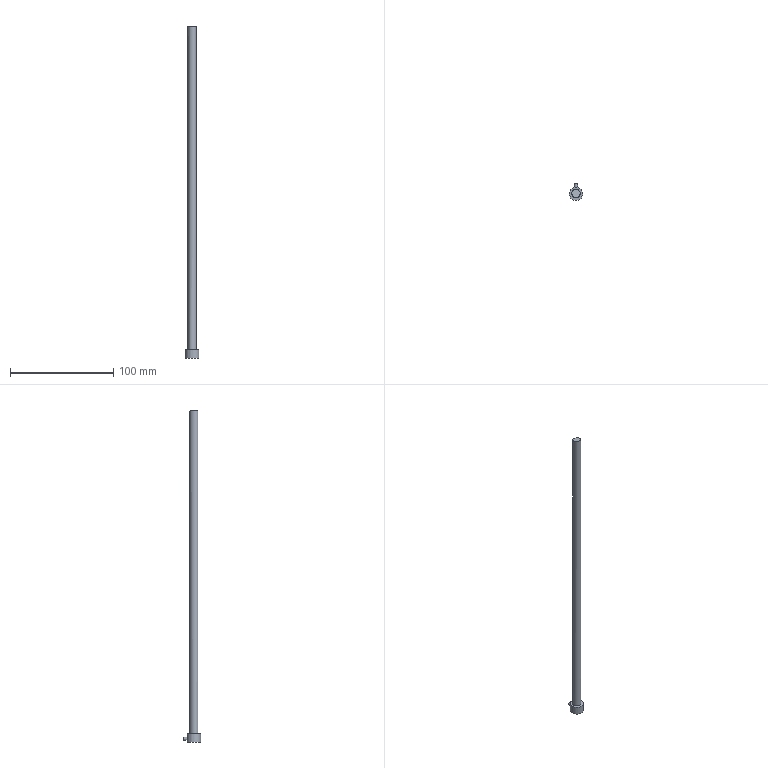Part | STEP file | E108-05-325 | 1 solid | 8 faces | box 13 x 16.5 x 321.213 mm | volume 16796 mm3 | cylinder 3 | plane 3 | spline 1 | cone 1 | commonest cylinder face diameters 3 x1 8 x1 13 x1
STEP:
#1=CARTESIAN_POINT('',(0.,0.,0.));
#2=DIRECTION('',(0.,0.,1.));
#3=DIRECTION('',(1.,0.,0.));
#4=AXIS2_PLACEMENT_3D('',#1,#2,#3);
#5=CARTESIAN_POINT('',(1.679,3.631,319.88));
#6=VERTEX_POINT('',#5);
#7=CARTESIAN_POINT('',(1.679,3.631,319.88));
#8=CARTESIAN_POINT('',(1.275,3.818,319.887));
#9=CARTESIAN_POINT('',(0.833,3.937,319.907));
#10=CARTESIAN_POINT('',(0.3906,3.981,319.935));
#11=CARTESIAN_POINT('',(-0.05165,4.024,319.963));
#12=CARTESIAN_POINT('',(-0.5067,3.992,320.));
#13=CARTESIAN_POINT('',(-0.9375,3.889,320.044));
#14=CARTESIAN_POINT('',(-1.371,3.784,320.089));
#15=CARTESIAN_POINT('',(-1.791,3.604,320.141));
#16=CARTESIAN_POINT('',(-2.165,3.363,320.197));
#17=CARTESIAN_POINT('',(-2.542,3.121,320.253));
#18=CARTESIAN_POINT('',(-2.882,2.81,320.316));
#19=CARTESIAN_POINT('',(-3.157,2.457,320.38));
#20=CARTESIAN_POINT('',(-3.433,2.101,320.445));
#21=CARTESIAN_POINT('',(-3.652,1.693,320.514));
#22=CARTESIAN_POINT('',(-3.794,1.266,320.582));
#23=CARTESIAN_POINT('',(-3.938,0.837,320.65));
#24=CARTESIAN_POINT('',(-4.008,0.3771,320.72));
#25=CARTESIAN_POINT('',(-3.999,-0.07547,320.786));
#26=CARTESIAN_POINT('',(-3.991,-0.5283,320.852));
#27=CARTESIAN_POINT('',(-3.903,-0.9864,320.916));
#28=CARTESIAN_POINT('',(-3.743,-1.411,320.973));
#29=CARTESIAN_POINT('',(-3.583,-1.834,321.029));
#30=CARTESIAN_POINT('',(-3.348,-2.236,321.08));
#31=CARTESIAN_POINT('',(-3.055,-2.582,321.119));
#32=CARTESIAN_POINT('',(-2.765,-2.925,321.158));
#33=CARTESIAN_POINT('',(-2.411,-3.223,321.187));
#34=CARTESIAN_POINT('',(-2.023,-3.451,321.201));
#35=CARTESIAN_POINT('',(-1.64,-3.675,321.216));
#36=CARTESIAN_POINT('',(-1.213,-3.837,321.217));
#37=CARTESIAN_POINT('',(-0.778,-3.924,321.204));
#38=CARTESIAN_POINT('',(-0.3463,-4.009,321.191));
#39=CARTESIAN_POINT('',(0.1053,-4.023,321.163));
#40=CARTESIAN_POINT('',(0.5397,-3.963,321.123));
#41=CARTESIAN_POINT('',(0.9755,-3.904,321.083));
#42=CARTESIAN_POINT('',(1.406,-3.77,321.029));
#43=CARTESIAN_POINT('',(1.796,-3.574,320.967));
#44=CARTESIAN_POINT('',(2.193,-3.375,320.903));
#45=CARTESIAN_POINT('',(2.56,-3.105,320.829));
#46=CARTESIAN_POINT('',(2.867,-2.789,320.751));
#47=CARTESIAN_POINT('',(3.181,-2.466,320.672));
#48=CARTESIAN_POINT('',(3.443,-2.085,320.588));
#49=CARTESIAN_POINT('',(3.631,-1.677,320.506));
#50=CARTESIAN_POINT('',(3.822,-1.264,320.423));
#51=CARTESIAN_POINT('',(3.943,-0.8121,320.34));
#52=CARTESIAN_POINT('',(3.984,-0.3577,320.266));
#53=CARTESIAN_POINT('',(4.025,0.09521,320.191));
#54=CARTESIAN_POINT('',(3.987,0.563,320.123));
#55=CARTESIAN_POINT('',(3.872,1.006,320.067));
#56=CARTESIAN_POINT('',(3.758,1.442,320.012));
#57=CARTESIAN_POINT('',(3.567,1.866,319.967));
#58=CARTESIAN_POINT('',(3.313,2.241,319.936));
#59=CARTESIAN_POINT('',(3.063,2.611,319.904));
#60=CARTESIAN_POINT('',(2.746,2.943,319.885));
#61=CARTESIAN_POINT('',(2.387,3.209,319.879));
#62=CARTESIAN_POINT('',(2.167,3.373,319.875));
#63=CARTESIAN_POINT('',(1.928,3.515,319.875));
#64=CARTESIAN_POINT('',(1.679,3.631,319.88));
#65=B_SPLINE_CURVE_WITH_KNOTS('',3,(#7,#8,#9,#10,#11,#12,#13,#14,#15,#16,#17,#18,#19,#20,#21,#22,#23,#24,#25,#26,#27,#28,#29,#30,#31,#32,#33,#34,#35,#36,#37,#38,#39,#40,#41,#42,#43,#44,#45,#46,#47,#48,#49,#50,#51,#52,#53,#54,#55,#56,#57,#58,#59,#60,#61,#62,#63,#64),.UNSPECIFIED.,.T.,.F.,(1,3,3,3,3,3,3,3,3,3,3,3,3,3,3,3,3,3,3,3,3,1),(-0.03244,0.,0.05305,0.1061,0.1594,0.2133,0.2675,0.322,0.3766,0.4308,0.4845,0.5374,0.5898,0.6424,0.6958,0.7502,0.8053,0.8602,0.9143,0.9676,1.,1.053),.UNSPECIFIED.);
#66=CARTESIAN_POINT('',(0.,0.,108.));
#67=DIRECTION('',(0.,0.,-1.));
#68=DIRECTION('',(-1.,0.,0.));
#69=AXIS2_PLACEMENT_3D('',#66,#67,#68);
#70=CYLINDRICAL_SURFACE('',#69,4.);
#71=CARTESIAN_POINT('',(8.287,-211.88));
#72=CARTESIAN_POINT('',(8.263,-211.881));
#73=CARTESIAN_POINT('',(8.215,-211.886));
#74=CARTESIAN_POINT('',(8.143,-211.895));
#75=CARTESIAN_POINT('',(8.071,-211.908));
#76=CARTESIAN_POINT('',(8.,-211.923));
#77=CARTESIAN_POINT('',(7.928,-211.94));
#78=CARTESIAN_POINT('',(7.856,-211.96));
#79=CARTESIAN_POINT('',(7.785,-211.983));
#80=CARTESIAN_POINT('',(7.713,-212.008));
#81=CARTESIAN_POINT('',(7.641,-212.034));
#82=CARTESIAN_POINT('',(7.57,-212.063));
#83=CARTESIAN_POINT('',(7.499,-212.094));
#84=CARTESIAN_POINT('',(7.427,-212.126));
#85=CARTESIAN_POINT('',(7.355,-212.16));
#86=CARTESIAN_POINT('',(7.284,-212.195));
#87=CARTESIAN_POINT('',(7.213,-212.232));
#88=CARTESIAN_POINT('',(7.142,-212.27));
#89=CARTESIAN_POINT('',(7.07,-212.309));
#90=CARTESIAN_POINT('',(6.999,-212.349));
#91=CARTESIAN_POINT('',(6.928,-212.39));
#92=CARTESIAN_POINT('',(6.857,-212.431));
#93=CARTESIAN_POINT('',(6.786,-212.473));
#94=CARTESIAN_POINT('',(6.715,-212.516));
#95=CARTESIAN_POINT('',(6.643,-212.559));
#96=CARTESIAN_POINT('',(6.573,-212.602));
#97=CARTESIAN_POINT('',(6.502,-212.645));
#98=CARTESIAN_POINT('',(6.43,-212.688));
#99=CARTESIAN_POINT('',(6.359,-212.73));
#100=CARTESIAN_POINT('',(6.288,-212.772));
#101=CARTESIAN_POINT('',(6.217,-212.813));
#102=CARTESIAN_POINT('',(6.146,-212.854));
#103=CARTESIAN_POINT('',(6.075,-212.894));
#104=CARTESIAN_POINT('',(6.003,-212.932));
#105=CARTESIAN_POINT('',(5.932,-212.968));
#106=CARTESIAN_POINT('',(5.861,-213.003));
#107=CARTESIAN_POINT('',(5.79,-213.036));
#108=CARTESIAN_POINT('',(5.718,-213.067));
#109=CARTESIAN_POINT('',(5.646,-213.096));
#110=CARTESIAN_POINT('',(5.575,-213.122));
#111=CARTESIAN_POINT('',(5.504,-213.145));
#112=CARTESIAN_POINT('',(5.432,-213.165));
#113=CARTESIAN_POINT('',(5.36,-213.182));
#114=CARTESIAN_POINT('',(5.288,-213.195));
#115=CARTESIAN_POINT('',(5.216,-213.205));
#116=CARTESIAN_POINT('',(5.145,-213.211));
#117=CARTESIAN_POINT('',(5.073,-213.214));
#118=CARTESIAN_POINT('',(5.,-213.212));
#119=CARTESIAN_POINT('',(4.929,-213.207));
#120=CARTESIAN_POINT('',(4.857,-213.198));
#121=CARTESIAN_POINT('',(4.785,-213.184));
#122=CARTESIAN_POINT('',(4.713,-213.167));
#123=CARTESIAN_POINT('',(4.641,-213.146));
#124=CARTESIAN_POINT('',(4.57,-213.121));
#125=CARTESIAN_POINT('',(4.499,-213.093));
#126=CARTESIAN_POINT('',(4.427,-213.061));
#127=CARTESIAN_POINT('',(4.355,-213.026));
#128=CARTESIAN_POINT('',(4.284,-212.988));
#129=CARTESIAN_POINT('',(4.213,-212.948));
#130=CARTESIAN_POINT('',(4.142,-212.904));
#131=CARTESIAN_POINT('',(4.071,-212.859));
#132=CARTESIAN_POINT('',(4.,-212.812));
#133=CARTESIAN_POINT('',(3.929,-212.763));
#134=CARTESIAN_POINT('',(3.859,-212.713));
#135=CARTESIAN_POINT('',(3.788,-212.662));
#136=CARTESIAN_POINT('',(3.717,-212.61));
#137=CARTESIAN_POINT('',(3.646,-212.558));
#138=CARTESIAN_POINT('',(3.576,-212.507));
#139=CARTESIAN_POINT('',(3.505,-212.455));
#140=CARTESIAN_POINT('',(3.434,-212.404));
#141=CARTESIAN_POINT('',(3.363,-212.354));
#142=CARTESIAN_POINT('',(3.292,-212.306));
#143=CARTESIAN_POINT('',(3.222,-212.259));
#144=CARTESIAN_POINT('',(3.151,-212.214));
#145=CARTESIAN_POINT('',(3.08,-212.171));
#146=CARTESIAN_POINT('',(3.008,-212.13));
#147=CARTESIAN_POINT('',(2.937,-212.092));
#148=CARTESIAN_POINT('',(2.866,-212.056));
#149=CARTESIAN_POINT('',(2.795,-212.024));
#150=CARTESIAN_POINT('',(2.723,-211.994));
#151=CARTESIAN_POINT('',(2.651,-211.968));
#152=CARTESIAN_POINT('',(2.58,-211.944));
#153=CARTESIAN_POINT('',(2.508,-211.925));
#154=CARTESIAN_POINT('',(2.436,-211.908));
#155=CARTESIAN_POINT('',(2.365,-211.895));
#156=CARTESIAN_POINT('',(2.292,-211.885));
#157=CARTESIAN_POINT('',(2.221,-211.879));
#158=CARTESIAN_POINT('',(2.149,-211.876));
#159=CARTESIAN_POINT('',(2.076,-211.876));
#160=CARTESIAN_POINT('',(2.028,-211.878));
#161=CARTESIAN_POINT('',(2.004,-211.88));
#162=B_SPLINE_CURVE_WITH_KNOTS('',3,(#71,#72,#73,#74,#75,#76,#77,#78,#79,#80,#81,#82,#83,#84,#85,#86,#87,#88,#89,#90,#91,#92,#93,#94,#95,#96,#97,#98,#99,#100,#101,#102,#103,#104,#105,#106,#107,#108,#109,#110,#111,#112,#113,#114,#115,#116,#117,#118,#119,#120,#121,#122,#123,#124,#125,#126,#127,#128,#129,#130,#131,#132,#133,#134,#135,#136,#137,#138,#139,#140,#141,#142,#143,#144,#145,#146,#147,#148,#149,#150,#151,#152,#153,#154,#155,#156,#157,#158,#159,#160,#161),.UNSPECIFIED.,.F.,.F.,(4,1,1,1,1,1,1,1,1,1,1,1,1,1,1,1,1,1,1,1,1,1,1,1,1,1,1,1,1,1,1,1,1,1,1,1,1,1,1,1,1,1,1,1,1,1,1,1,1,1,1,1,1,1,1,1,1,1,1,1,1,1,1,1,1,1,1,1,1,1,1,1,1,1,1,1,1,1,1,1,1,1,1,1,1,1,1,1,4),(0.,0.01136,0.02273,0.03409,0.04545,0.05682,0.06818,0.07955,0.09091,0.1023,0.1136,0.125,0.1364,0.1477,0.1591,0.1705,0.1818,0.1932,0.2045,0.2159,0.2273,0.2386,0.25,0.2614,0.2727,0.2841,0.2955,0.3068,0.3182,0.3295,0.3409,0.3523,0.3636,0.375,0.3864,0.3977,0.4091,0.4205,0.4318,0.4432,0.4545,0.4659,0.4773,0.4886,0.5,0.5114,0.5227,0.5341,0.5455,0.5568,0.5682,0.5795,0.5909,0.6023,0.6136,0.625,0.6364,0.6477,0.6591,0.6705,0.6818,0.6932,0.7045,0.7159,0.7273,0.7386,0.75,0.7614,0.7727,0.7841,0.7955,0.8068,0.8182,0.8295,0.8409,0.8523,0.8636,0.875,0.8864,0.8977,0.9091,0.9205,0.9318,0.9432,0.9545,0.9659,0.9773,0.9886,1.),.QUASI_UNIFORM_KNOTS.);
#163=(GEOMETRIC_REPRESENTATION_CONTEXT(2)PARAMETRIC_REPRESENTATION_CONTEXT()REPRESENTATION_CONTEXT('',''));
#164=DEFINITIONAL_REPRESENTATION('',(#162),#163);
#165=PCURVE('',#70,#164);
#166=CARTESIAN_POINT('',(66.102,21.89,305.613));
#167=CARTESIAN_POINT('',(53.721,19.516,309.382));
#168=CARTESIAN_POINT('',(41.284,16.881,312.607));
#169=CARTESIAN_POINT('',(22.662,12.441,316.385));
#170=CARTESIAN_POINT('',(16.461,10.88,317.468));
#171=CARTESIAN_POINT('',(7.202,8.408,318.804));
#172=CARTESIAN_POINT('',(4.122,7.562,319.201));
#173=CARTESIAN_POINT('',(-0.4807,6.26,319.724));
#174=CARTESIAN_POINT('',(-2.012,5.82,319.886));
#175=CARTESIAN_POINT('',(-5.069,4.93,320.186));
#176=CARTESIAN_POINT('',(-6.578,4.483,320.322));
#177=CARTESIAN_POINT('',(-8.115,4.023,320.448));
#178=CARTESIAN_POINT('',(66.596,17.63,305.901));
#179=CARTESIAN_POINT('',(54.268,15.188,309.678));
#180=CARTESIAN_POINT('',(41.894,12.489,312.921));
#181=CARTESIAN_POINT('',(23.381,7.953,316.752));
#182=CARTESIAN_POINT('',(17.219,6.36,317.857));
#183=CARTESIAN_POINT('',(8.021,3.839,319.236));
#184=CARTESIAN_POINT('',(4.963,2.976,319.649));
#185=CARTESIAN_POINT('',(0.3919,1.65,320.198));
#186=CARTESIAN_POINT('',(-1.129,1.202,320.369));
#187=CARTESIAN_POINT('',(-4.164,0.2944,320.688));
#188=CARTESIAN_POINT('',(-5.663,-0.1618,320.834));
#189=CARTESIAN_POINT('',(-7.189,-0.6297,320.971));
#190=CARTESIAN_POINT('',(67.127,13.38,306.313));
#191=CARTESIAN_POINT('',(54.851,10.872,310.103));
#192=CARTESIAN_POINT('',(42.537,8.108,313.368));
#193=CARTESIAN_POINT('',(24.128,3.479,317.264));
#194=CARTESIAN_POINT('',(18.003,1.856,318.395));
#195=CARTESIAN_POINT('',(8.862,-0.7111,319.823));
#196=CARTESIAN_POINT('',(5.823,-1.589,320.254));
#197=CARTESIAN_POINT('',(1.282,-2.939,320.833));
#198=CARTESIAN_POINT('',(-0.2284,-3.394,321.015));
#199=CARTESIAN_POINT('',(-3.243,-4.317,321.355));
#200=CARTESIAN_POINT('',(-4.732,-4.781,321.513));
#201=CARTESIAN_POINT('',(-6.248,-5.256,321.662));
#202=CARTESIAN_POINT('',(67.706,9.139,306.89));
#203=CARTESIAN_POINT('',(55.479,6.564,310.696));
#204=CARTESIAN_POINT('',(43.222,3.737,313.989));
#205=CARTESIAN_POINT('',(24.909,-0.9819,317.959));
#206=CARTESIAN_POINT('',(18.818,-2.635,319.121));
#207=CARTESIAN_POINT('',(9.731,-5.245,320.604));
#208=CARTESIAN_POINT('',(6.71,-6.137,321.056));
#209=CARTESIAN_POINT('',(2.196,-7.508,321.668));
#210=CARTESIAN_POINT('',(0.6947,-7.971,321.861));
#211=CARTESIAN_POINT('',(-2.302,-8.907,322.225));
#212=CARTESIAN_POINT('',(-3.782,-9.379,322.396));
#213=CARTESIAN_POINT('',(-5.288,-9.861,322.558));
#214=B_SPLINE_SURFACE_WITH_KNOTS('',3,3,((#166,#167,#168,#169,#170,#171,#172,#173,#174,#175,#176,#177),(#178,#179,#180,#181,#182,#183,#184,#185,#186,#187,#188,#189),(#190,#191,#192,#193,#194,#195,#196,#197,#198,#199,#200,#201),(#202,#203,#204,#205,#206,#207,#208,#209,#210,#211,#212,#213)),.UNSPECIFIED.,.F.,.F.,.F.,(4,4),(4,2,2,2,2,4),(0.,1.),(0.,0.5,0.75,0.875,0.9375,1.),.UNSPECIFIED.);
#215=CARTESIAN_POINT('',(0.2231,0.8744));
#216=CARTESIAN_POINT('',(0.2186,0.8754));
#217=CARTESIAN_POINT('',(0.21,0.8775));
#218=CARTESIAN_POINT('',(0.1983,0.8808));
#219=CARTESIAN_POINT('',(0.1878,0.8842));
#220=CARTESIAN_POINT('',(0.1786,0.8878));
#221=CARTESIAN_POINT('',(0.1708,0.8914));
#222=CARTESIAN_POINT('',(0.1644,0.895));
#223=CARTESIAN_POINT('',(0.1593,0.8988));
#224=CARTESIAN_POINT('',(0.1557,0.9026));
#225=CARTESIAN_POINT('',(0.1535,0.9063));
#226=CARTESIAN_POINT('',(0.1528,0.9101));
#227=CARTESIAN_POINT('',(0.1536,0.9138));
#228=CARTESIAN_POINT('',(0.1558,0.9175));
#229=CARTESIAN_POINT('',(0.1594,0.9211));
#230=CARTESIAN_POINT('',(0.1644,0.9247));
#231=CARTESIAN_POINT('',(0.1708,0.9281));
#232=CARTESIAN_POINT('',(0.1786,0.9314));
#233=CARTESIAN_POINT('',(0.1876,0.9346));
#234=CARTESIAN_POINT('',(0.1979,0.9377));
#235=CARTESIAN_POINT('',(0.2093,0.9405));
#236=CARTESIAN_POINT('',(0.2219,0.9432));
#237=CARTESIAN_POINT('',(0.2357,0.9458));
#238=CARTESIAN_POINT('',(0.2504,0.9481));
#239=CARTESIAN_POINT('',(0.2661,0.9502));
#240=CARTESIAN_POINT('',(0.2825,0.952));
#241=CARTESIAN_POINT('',(0.2998,0.9537));
#242=CARTESIAN_POINT('',(0.3178,0.9551));
#243=CARTESIAN_POINT('',(0.3365,0.9562));
#244=CARTESIAN_POINT('',(0.3556,0.9571));
#245=CARTESIAN_POINT('',(0.375,0.9577));
#246=CARTESIAN_POINT('',(0.395,0.9581));
#247=CARTESIAN_POINT('',(0.4151,0.9582));
#248=CARTESIAN_POINT('',(0.4354,0.958));
#249=CARTESIAN_POINT('',(0.4557,0.9575));
#250=CARTESIAN_POINT('',(0.4759,0.9568));
#251=CARTESIAN_POINT('',(0.496,0.9558));
#252=CARTESIAN_POINT('',(0.5159,0.9546));
#253=CARTESIAN_POINT('',(0.5354,0.9531));
#254=CARTESIAN_POINT('',(0.5543,0.9514));
#255=CARTESIAN_POINT('',(0.5727,0.9494));
#256=CARTESIAN_POINT('',(0.5905,0.9472));
#257=CARTESIAN_POINT('',(0.6076,0.9447));
#258=CARTESIAN_POINT('',(0.6238,0.9421));
#259=CARTESIAN_POINT('',(0.6389,0.9393));
#260=CARTESIAN_POINT('',(0.6532,0.9363));
#261=CARTESIAN_POINT('',(0.6663,0.9331));
#262=CARTESIAN_POINT('',(0.6783,0.9298));
#263=CARTESIAN_POINT('',(0.689,0.9263));
#264=CARTESIAN_POINT('',(0.6984,0.9228));
#265=CARTESIAN_POINT('',(0.7065,0.9192));
#266=CARTESIAN_POINT('',(0.7132,0.9154));
#267=CARTESIAN_POINT('',(0.7185,0.9117));
#268=CARTESIAN_POINT('',(0.7223,0.9079));
#269=CARTESIAN_POINT('',(0.7247,0.9041));
#270=CARTESIAN_POINT('',(0.7256,0.9003));
#271=CARTESIAN_POINT('',(0.725,0.8965));
#272=CARTESIAN_POINT('',(0.723,0.8928));
#273=CARTESIAN_POINT('',(0.7195,0.8892));
#274=CARTESIAN_POINT('',(0.7145,0.8856));
#275=CARTESIAN_POINT('',(0.7082,0.8822));
#276=CARTESIAN_POINT('',(0.7005,0.8788));
#277=CARTESIAN_POINT('',(0.6915,0.8756));
#278=CARTESIAN_POINT('',(0.6813,0.8726));
#279=CARTESIAN_POINT('',(0.6697,0.8697));
#280=CARTESIAN_POINT('',(0.657,0.867));
#281=CARTESIAN_POINT('',(0.6432,0.8645));
#282=CARTESIAN_POINT('',(0.6285,0.8622));
#283=CARTESIAN_POINT('',(0.6127,0.8601));
#284=CARTESIAN_POINT('',(0.5961,0.8583));
#285=CARTESIAN_POINT('',(0.5786,0.8567));
#286=CARTESIAN_POINT('',(0.5604,0.8553));
#287=CARTESIAN_POINT('',(0.5416,0.8542));
#288=CARTESIAN_POINT('',(0.5223,0.8533));
#289=CARTESIAN_POINT('',(0.5025,0.8527));
#290=CARTESIAN_POINT('',(0.4823,0.8523));
#291=CARTESIAN_POINT('',(0.4619,0.8523));
#292=CARTESIAN_POINT('',(0.4415,0.8525));
#293=CARTESIAN_POINT('',(0.421,0.8529));
#294=CARTESIAN_POINT('',(0.4005,0.8537));
#295=CARTESIAN_POINT('',(0.3802,0.8547));
#296=CARTESIAN_POINT('',(0.3602,0.8559));
#297=CARTESIAN_POINT('',(0.3407,0.8574));
#298=CARTESIAN_POINT('',(0.3216,0.8592));
#299=CARTESIAN_POINT('',(0.3031,0.8612));
#300=CARTESIAN_POINT('',(0.2853,0.8634));
#301=CARTESIAN_POINT('',(0.2684,0.8658));
#302=CARTESIAN_POINT('',(0.2522,0.8685));
#303=CARTESIAN_POINT('',(0.237,0.8713));
#304=CARTESIAN_POINT('',(0.2276,0.8733));
#305=CARTESIAN_POINT('',(0.2231,0.8744));
#306=B_SPLINE_CURVE_WITH_KNOTS('',3,(#215,#216,#217,#218,#219,#220,#221,#222,#223,#224,#225,#226,#227,#228,#229,#230,#231,#232,#233,#234,#235,#236,#237,#238,#239,#240,#241,#242,#243,#244,#245,#246,#247,#248,#249,#250,#251,#252,#253,#254,#255,#256,#257,#258,#259,#260,#261,#262,#263,#264,#265,#266,#267,#268,#269,#270,#271,#272,#273,#274,#275,#276,#277,#278,#279,#280,#281,#282,#283,#284,#285,#286,#287,#288,#289,#290,#291,#292,#293,#294,#295,#296,#297,#298,#299,#300,#301,#302,#303,#304,#305),.UNSPECIFIED.,.T.,.F.,(4,1,1,1,1,1,1,1,1,1,1,1,1,1,1,1,1,1,1,1,1,1,1,1,1,1,1,1,1,1,1,1,1,1,1,1,1,1,1,1,1,1,1,1,1,1,1,1,1,1,1,1,1,1,1,1,1,1,1,1,1,1,1,1,1,1,1,1,1,1,1,1,1,1,1,1,1,1,1,1,1,1,1,1,1,1,1,1,4),(0.,0.01136,0.02273,0.03409,0.04545,0.05682,0.06818,0.07955,0.09091,0.1023,0.1136,0.125,0.1364,0.1477,0.1591,0.1705,0.1818,0.1932,0.2045,0.2159,0.2273,0.2386,0.25,0.2614,0.2727,0.2841,0.2955,0.3068,0.3182,0.3295,0.3409,0.3523,0.3636,0.375,0.3864,0.3977,0.4091,0.4205,0.4318,0.4432,0.4545,0.4659,0.4773,0.4886,0.5,0.5114,0.5227,0.5341,0.5455,0.5568,0.5682,0.5795,0.5909,0.6023,0.6136,0.625,0.6364,0.6477,0.6591,0.6705,0.6818,0.6932,0.7045,0.7159,0.7273,0.7386,0.75,0.7614,0.7727,0.7841,0.7955,0.8068,0.8182,0.8295,0.8409,0.8523,0.8636,0.875,0.8864,0.8977,0.9091,0.9205,0.9318,0.9432,0.9545,0.9659,0.9773,0.9886,1.),.QUASI_UNIFORM_KNOTS.);
#307=(GEOMETRIC_REPRESENTATION_CONTEXT(2)PARAMETRIC_REPRESENTATION_CONTEXT()REPRESENTATION_CONTEXT('',''));
#308=DEFINITIONAL_REPRESENTATION('',(#306),#307);
#309=PCURVE('',#214,#308);
#310=SURFACE_CURVE('',#65,(#165,#309),.PCURVE_S1.);
#311=EDGE_CURVE('',#6,#6,#310,.T.);
#312=ORIENTED_EDGE('',*,*,#311,.F.);
#313=CARTESIAN_POINT('',(1.679,3.631,8.));
#314=VERTEX_POINT('',#313);
#315=CARTESIAN_POINT('',(1.679,3.631,319.88));
#316=CARTESIAN_POINT('',(1.679,3.631,8.));
#317=B_SPLINE_CURVE_WITH_KNOTS('',1,(#315,#316),.UNSPECIFIED.,.F.,.F.,(2,2),(-211.88,100.),.PIECEWISE_BEZIER_KNOTS.);
#318=CARTESIAN_POINT('',(8.287,0.));
#319=DIRECTION('',(0.,1.));
#320=VECTOR('',#319,1.);
#321=LINE('',#318,#320);
#322=(GEOMETRIC_REPRESENTATION_CONTEXT(2)PARAMETRIC_REPRESENTATION_CONTEXT()REPRESENTATION_CONTEXT('',''));
#323=DEFINITIONAL_REPRESENTATION('',(#321),#322);
#324=PCURVE('',#70,#323);
#325=CARTESIAN_POINT('',(2.004,0.));
#326=DIRECTION('',(0.,1.));
#327=VECTOR('',#326,1.);
#328=LINE('',#325,#327);
#329=(GEOMETRIC_REPRESENTATION_CONTEXT(2)PARAMETRIC_REPRESENTATION_CONTEXT()REPRESENTATION_CONTEXT('',''));
#330=DEFINITIONAL_REPRESENTATION('',(#328),#329);
#331=PCURVE('',#70,#330);
#332=SEAM_CURVE('',#317,(#324,#331),.PCURVE_S1.);
#333=EDGE_CURVE('',#6,#314,#332,.T.);
#334=ORIENTED_EDGE('',*,*,#333,.T.);
#335=CARTESIAN_POINT('',(4.,0.,8.));
#336=VERTEX_POINT('',#335);
#337=CARTESIAN_POINT('',(0.,0.,8.));
#338=DIRECTION('',(0.,0.,1.));
#339=DIRECTION('',(1.,0.,0.));
#340=AXIS2_PLACEMENT_3D('',#337,#338,#339);
#341=CIRCLE('',#340,4.);
#342=CARTESIAN_POINT('',(9.425,100.));
#343=DIRECTION('',(-1.,0.));
#344=VECTOR('',#343,1.);
#345=LINE('',#342,#344);
#346=(GEOMETRIC_REPRESENTATION_CONTEXT(2)PARAMETRIC_REPRESENTATION_CONTEXT()REPRESENTATION_CONTEXT('',''));
#347=DEFINITIONAL_REPRESENTATION('',(#345),#346);
#348=PCURVE('',#70,#347);
#349=CARTESIAN_POINT('',(0.,0.,8.));
#350=DIRECTION('',(0.,0.,-1.));
#351=DIRECTION('',(1.,0.,0.));
#352=AXIS2_PLACEMENT_3D('',#349,#350,#351);
#353=PLANE('',#352);
#354=CARTESIAN_POINT('',(4.,0.));
#355=CARTESIAN_POINT('',(4.,-6.928));
#356=CARTESIAN_POINT('',(-2.,-3.464));
#357=CARTESIAN_POINT('',(-8.,0.));
#358=CARTESIAN_POINT('',(-2.,3.464));
#359=CARTESIAN_POINT('',(4.,6.928));
#360=CARTESIAN_POINT('',(4.,0.));
#361=(BOUNDED_CURVE()B_SPLINE_CURVE(2,(#354,#355,#356,#357,#358,#359,#360),.UNSPECIFIED.,.T.,.F.)B_SPLINE_CURVE_WITH_KNOTS((1,2,2,2,2,1),(-2.094,0.,2.094,4.189,6.283,8.378),.UNSPECIFIED.)CURVE()GEOMETRIC_REPRESENTATION_ITEM()RATIONAL_B_SPLINE_CURVE((1.,0.5,1.,0.5,1.,0.5,1.))REPRESENTATION_ITEM(''));
#362=(GEOMETRIC_REPRESENTATION_CONTEXT(2)PARAMETRIC_REPRESENTATION_CONTEXT()REPRESENTATION_CONTEXT('',''));
#363=DEFINITIONAL_REPRESENTATION('',(#361),#362);
#364=PCURVE('',#353,#363);
#365=SURFACE_CURVE('',#341,(#348,#364),.PCURVE_S1.);
#366=EDGE_CURVE('',#314,#336,#365,.T.);
#367=ORIENTED_EDGE('',*,*,#366,.T.);
#368=CARTESIAN_POINT('',(0.,0.,8.));
#369=DIRECTION('',(0.,0.,1.));
#370=DIRECTION('',(1.,0.,0.));
#371=AXIS2_PLACEMENT_3D('',#368,#369,#370);
#372=CIRCLE('',#371,4.);
#373=CARTESIAN_POINT('',(3.142,100.));
#374=DIRECTION('',(-1.,0.));
#375=VECTOR('',#374,1.);
#376=LINE('',#373,#375);
#377=(GEOMETRIC_REPRESENTATION_CONTEXT(2)PARAMETRIC_REPRESENTATION_CONTEXT()REPRESENTATION_CONTEXT('',''));
#378=DEFINITIONAL_REPRESENTATION('',(#376),#377);
#379=PCURVE('',#70,#378);
#380=CARTESIAN_POINT('',(4.,0.));
#381=CARTESIAN_POINT('',(4.,-6.928));
#382=CARTESIAN_POINT('',(-2.,-3.464));
#383=CARTESIAN_POINT('',(-8.,0.));
#384=CARTESIAN_POINT('',(-2.,3.464));
#385=CARTESIAN_POINT('',(4.,6.928));
#386=CARTESIAN_POINT('',(4.,0.));
#387=(BOUNDED_CURVE()B_SPLINE_CURVE(2,(#380,#381,#382,#383,#384,#385,#386),.UNSPECIFIED.,.T.,.F.)B_SPLINE_CURVE_WITH_KNOTS((1,2,2,2,2,1),(-2.094,0.,2.094,4.189,6.283,8.378),.UNSPECIFIED.)CURVE()GEOMETRIC_REPRESENTATION_ITEM()RATIONAL_B_SPLINE_CURVE((1.,0.5,1.,0.5,1.,0.5,1.))REPRESENTATION_ITEM(''));
#388=(GEOMETRIC_REPRESENTATION_CONTEXT(2)PARAMETRIC_REPRESENTATION_CONTEXT()REPRESENTATION_CONTEXT('',''));
#389=DEFINITIONAL_REPRESENTATION('',(#387),#388);
#390=PCURVE('',#353,#389);
#391=SURFACE_CURVE('',#372,(#379,#390),.PCURVE_S1.);
#392=EDGE_CURVE('',#336,#314,#391,.T.);
#393=ORIENTED_EDGE('',*,*,#392,.T.);
#394=ORIENTED_EDGE('',*,*,#333,.F.);
#395=EDGE_LOOP('',(#312,#334,#367,#393,#394));
#396=FACE_BOUND('',#395,.T.);
#397=ADVANCED_FACE('',(#396),#70,.T.);
#398=ORIENTED_EDGE('',*,*,#311,.F.);
#399=EDGE_LOOP('',(#398));
#400=FACE_BOUND('',#399,.F.);
#401=ADVANCED_FACE('',(#400),#214,.F.);
#402=CARTESIAN_POINT('',(6.5,0.,0.));
#403=VERTEX_POINT('',#402);
#404=CARTESIAN_POINT('',(-6.5,0.,0.));
#405=VERTEX_POINT('',#404);
#406=CARTESIAN_POINT('',(0.,0.,0.));
#407=DIRECTION('',(0.,0.,-1.));
#408=DIRECTION('',(-1.,0.,0.));
#409=AXIS2_PLACEMENT_3D('',#406,#407,#408);
#410=CIRCLE('',#409,6.5);
#411=CARTESIAN_POINT('',(0.,0.,8.));
#412=DIRECTION('',(0.,0.,-1.));
#413=DIRECTION('',(1.,0.,0.));
#414=AXIS2_PLACEMENT_3D('',#411,#412,#413);
#415=CYLINDRICAL_SURFACE('',#414,6.5);
#416=CARTESIAN_POINT('',(-3.142,8.));
#417=DIRECTION('',(1.,0.));
#418=VECTOR('',#417,1.);
#419=LINE('',#416,#418);
#420=(GEOMETRIC_REPRESENTATION_CONTEXT(2)PARAMETRIC_REPRESENTATION_CONTEXT()REPRESENTATION_CONTEXT('',''));
#421=DEFINITIONAL_REPRESENTATION('',(#419),#420);
#422=PCURVE('',#415,#421);
#423=CARTESIAN_POINT('',(240.,-1000.,0.));
#424=DIRECTION('',(0.,0.,1.));
#425=DIRECTION('',(-1.,0.,0.));
#426=AXIS2_PLACEMENT_3D('',#423,#424,#425);
#427=PLANE('',#426);
#428=CARTESIAN_POINT('',(246.5,-1000.));
#429=CARTESIAN_POINT('',(246.5,-1011.258));
#430=CARTESIAN_POINT('',(236.75,-1005.629));
#431=CARTESIAN_POINT('',(227.,-1000.));
#432=CARTESIAN_POINT('',(236.75,-994.371));
#433=CARTESIAN_POINT('',(246.5,-988.742));
#434=CARTESIAN_POINT('',(246.5,-1000.));
#435=(BOUNDED_CURVE()B_SPLINE_CURVE(2,(#428,#429,#430,#431,#432,#433,#434),.UNSPECIFIED.,.T.,.F.)B_SPLINE_CURVE_WITH_KNOTS((1,2,2,2,2,1),(-2.094,0.,2.094,4.189,6.283,8.378),.UNSPECIFIED.)CURVE()GEOMETRIC_REPRESENTATION_ITEM()RATIONAL_B_SPLINE_CURVE((1.,0.5,1.,0.5,1.,0.5,1.))REPRESENTATION_ITEM(''));
#436=(GEOMETRIC_REPRESENTATION_CONTEXT(2)PARAMETRIC_REPRESENTATION_CONTEXT()REPRESENTATION_CONTEXT('',''));
#437=DEFINITIONAL_REPRESENTATION('',(#435),#436);
#438=PCURVE('',#427,#437);
#439=SURFACE_CURVE('',#410,(#422,#438),.PCURVE_S1.);
#440=EDGE_CURVE('',#403,#405,#439,.T.);
#441=ORIENTED_EDGE('',*,*,#440,.F.);
#442=CARTESIAN_POINT('',(6.5,0.,8.));
#443=VERTEX_POINT('',#442);
#444=CARTESIAN_POINT('',(6.5,0.,8.));
#445=CARTESIAN_POINT('',(6.5,0.,0.));
#446=B_SPLINE_CURVE_WITH_KNOTS('',1,(#444,#445),.UNSPECIFIED.,.F.,.F.,(2,2),(0.,8.),.PIECEWISE_BEZIER_KNOTS.);
#447=CARTESIAN_POINT('',(0.,0.));
#448=DIRECTION('',(0.,1.));
#449=VECTOR('',#448,1.);
#450=LINE('',#447,#449);
#451=(GEOMETRIC_REPRESENTATION_CONTEXT(2)PARAMETRIC_REPRESENTATION_CONTEXT()REPRESENTATION_CONTEXT('',''));
#452=DEFINITIONAL_REPRESENTATION('',(#450),#451);
#453=PCURVE('',#415,#452);
#454=CARTESIAN_POINT('',(6.283,0.));
#455=DIRECTION('',(0.,1.));
#456=VECTOR('',#455,1.);
#457=LINE('',#454,#456);
#458=(GEOMETRIC_REPRESENTATION_CONTEXT(2)PARAMETRIC_REPRESENTATION_CONTEXT()REPRESENTATION_CONTEXT('',''));
#459=DEFINITIONAL_REPRESENTATION('',(#457),#458);
#460=PCURVE('',#415,#459);
#461=SEAM_CURVE('',#446,(#453,#460),.PCURVE_S1.);
#462=EDGE_CURVE('',#443,#403,#461,.T.);
#463=ORIENTED_EDGE('',*,*,#462,.F.);
#464=CARTESIAN_POINT('',(0.,0.,8.));
#465=DIRECTION('',(0.,0.,-1.));
#466=DIRECTION('',(1.,0.,0.));
#467=AXIS2_PLACEMENT_3D('',#464,#465,#466);
#468=CIRCLE('',#467,6.5);
#469=CARTESIAN_POINT('',(0.,0.));
#470=DIRECTION('',(1.,0.));
#471=VECTOR('',#470,1.);
#472=LINE('',#469,#471);
#473=(GEOMETRIC_REPRESENTATION_CONTEXT(2)PARAMETRIC_REPRESENTATION_CONTEXT()REPRESENTATION_CONTEXT('',''));
#474=DEFINITIONAL_REPRESENTATION('',(#472),#473);
#475=PCURVE('',#415,#474);
#476=CARTESIAN_POINT('',(0.,0.));
#477=DIRECTION('',(1.,0.));
#478=AXIS2_PLACEMENT_2D('',#476,#477);
#479=CIRCLE('',#478,6.5);
#480=(GEOMETRIC_REPRESENTATION_CONTEXT(2)PARAMETRIC_REPRESENTATION_CONTEXT()REPRESENTATION_CONTEXT('',''));
#481=DEFINITIONAL_REPRESENTATION('',(#479),#480);
#482=PCURVE('',#353,#481);
#483=SURFACE_CURVE('',#468,(#475,#482),.PCURVE_S1.);
#484=EDGE_CURVE('',#443,#443,#483,.T.);
#485=ORIENTED_EDGE('',*,*,#484,.T.);
#486=ORIENTED_EDGE('',*,*,#462,.T.);
#487=CARTESIAN_POINT('',(0.,0.,0.));
#488=DIRECTION('',(0.,0.,-1.));
#489=DIRECTION('',(-1.,0.,0.));
#490=AXIS2_PLACEMENT_3D('',#487,#488,#489);
#491=CIRCLE('',#490,6.5);
#492=CARTESIAN_POINT('',(3.142,8.));
#493=DIRECTION('',(1.,0.));
#494=VECTOR('',#493,1.);
#495=LINE('',#492,#494);
#496=(GEOMETRIC_REPRESENTATION_CONTEXT(2)PARAMETRIC_REPRESENTATION_CONTEXT()REPRESENTATION_CONTEXT('',''));
#497=DEFINITIONAL_REPRESENTATION('',(#495),#496);
#498=PCURVE('',#415,#497);
#499=CARTESIAN_POINT('',(246.5,-1000.));
#500=CARTESIAN_POINT('',(246.5,-1011.258));
#501=CARTESIAN_POINT('',(236.75,-1005.629));
#502=CARTESIAN_POINT('',(227.,-1000.));
#503=CARTESIAN_POINT('',(236.75,-994.371));
#504=CARTESIAN_POINT('',(246.5,-988.742));
#505=CARTESIAN_POINT('',(246.5,-1000.));
#506=(BOUNDED_CURVE()B_SPLINE_CURVE(2,(#499,#500,#501,#502,#503,#504,#505),.UNSPECIFIED.,.T.,.F.)B_SPLINE_CURVE_WITH_KNOTS((1,2,2,2,2,1),(-2.094,0.,2.094,4.189,6.283,8.378),.UNSPECIFIED.)CURVE()GEOMETRIC_REPRESENTATION_ITEM()RATIONAL_B_SPLINE_CURVE((1.,0.5,1.,0.5,1.,0.5,1.))REPRESENTATION_ITEM(''));
#507=(GEOMETRIC_REPRESENTATION_CONTEXT(2)PARAMETRIC_REPRESENTATION_CONTEXT()REPRESENTATION_CONTEXT('',''));
#508=DEFINITIONAL_REPRESENTATION('',(#506),#507);
#509=PCURVE('',#427,#508);
#510=SURFACE_CURVE('',#491,(#498,#509),.PCURVE_S1.);
#511=EDGE_CURVE('',#405,#403,#510,.T.);
#512=ORIENTED_EDGE('',*,*,#511,.F.);
#513=EDGE_LOOP('',(#441,#463,#485,#486,#512));
#514=FACE_BOUND('',#513,.T.);
#515=CARTESIAN_POINT('',(0.,6.5,1.5));
#516=VERTEX_POINT('',#515);
#517=CARTESIAN_POINT('',(0.,6.5,1.5));
#518=CARTESIAN_POINT('',(0.1654,6.5,1.5));
#519=CARTESIAN_POINT('',(0.3332,6.493,1.528));
#520=CARTESIAN_POINT('',(0.4892,6.482,1.582));
#521=CARTESIAN_POINT('',(0.6451,6.47,1.636));
#522=CARTESIAN_POINT('',(0.7936,6.453,1.717));
#523=CARTESIAN_POINT('',(0.9231,6.434,1.818));
#524=CARTESIAN_POINT('',(1.055,6.415,1.92));
#525=CARTESIAN_POINT('',(1.17,6.394,2.047));
#526=CARTESIAN_POINT('',(1.261,6.377,2.187));
#527=CARTESIAN_POINT('',(1.352,6.358,2.329));
#528=CARTESIAN_POINT('',(1.421,6.343,2.49));
#529=CARTESIAN_POINT('',(1.46,6.334,2.655));
#530=CARTESIAN_POINT('',(1.498,6.325,2.817));
#531=CARTESIAN_POINT('',(1.509,6.322,2.989));
#532=CARTESIAN_POINT('',(1.492,6.326,3.155));
#533=CARTESIAN_POINT('',(1.475,6.33,3.318));
#534=CARTESIAN_POINT('',(1.431,6.341,3.48));
#535=CARTESIAN_POINT('',(1.362,6.356,3.628));
#536=CARTESIAN_POINT('',(1.293,6.37,3.777));
#537=CARTESIAN_POINT('',(1.199,6.39,3.917));
#538=CARTESIAN_POINT('',(1.085,6.409,4.035));
#539=CARTESIAN_POINT('',(0.9695,6.428,4.157));
#540=CARTESIAN_POINT('',(0.8309,6.448,4.26));
#541=CARTESIAN_POINT('',(0.6809,6.464,4.337));
#542=CARTESIAN_POINT('',(0.5305,6.48,4.413));
#543=CARTESIAN_POINT('',(0.3642,6.492,4.465));
#544=CARTESIAN_POINT('',(0.1962,6.497,4.487));
#545=CARTESIAN_POINT('',(0.03191,6.502,4.509));
#546=CARTESIAN_POINT('',(-0.1386,6.501,4.503));
#547=CARTESIAN_POINT('',(-0.3008,6.493,4.47));
#548=CARTESIAN_POINT('',(-0.4611,6.486,4.437));
#549=CARTESIAN_POINT('',(-0.6177,6.472,4.377));
#550=CARTESIAN_POINT('',(-0.7583,6.456,4.294));
#551=CARTESIAN_POINT('',(-0.9011,6.439,4.211));
#552=CARTESIAN_POINT('',(-1.031,6.419,4.102));
#553=CARTESIAN_POINT('',(-1.139,6.399,3.976));
#554=CARTESIAN_POINT('',(-1.249,6.38,3.848));
#555=CARTESIAN_POINT('',(-1.338,6.361,3.699));
#556=CARTESIAN_POINT('',(-1.399,6.348,3.541));
#557=CARTESIAN_POINT('',(-1.46,6.334,3.384));
#558=CARTESIAN_POINT('',(-1.494,6.326,3.214));
#559=CARTESIAN_POINT('',(-1.499,6.325,3.046));
#560=CARTESIAN_POINT('',(-1.504,6.324,2.881));
#561=CARTESIAN_POINT('',(-1.482,6.329,2.714));
#562=CARTESIAN_POINT('',(-1.433,6.34,2.557));
#563=CARTESIAN_POINT('',(-1.385,6.351,2.4));
#564=CARTESIAN_POINT('',(-1.309,6.367,2.25));
#565=CARTESIAN_POINT('',(-1.214,6.386,2.119));
#566=CARTESIAN_POINT('',(-1.116,6.404,1.984));
#567=CARTESIAN_POINT('',(-0.9937,6.425,1.864));
#568=CARTESIAN_POINT('',(-0.8569,6.443,1.769));
#569=CARTESIAN_POINT('',(-0.7182,6.462,1.672));
#570=CARTESIAN_POINT('',(-0.5604,6.478,1.598));
#571=CARTESIAN_POINT('',(-0.3967,6.488,1.553));
#572=CARTESIAN_POINT('',(-0.2682,6.496,1.518));
#573=CARTESIAN_POINT('',(-0.1335,6.5,1.5));
#574=CARTESIAN_POINT('',(0.,6.5,1.5));
#575=B_SPLINE_CURVE_WITH_KNOTS('',3,(#517,#518,#519,#520,#521,#522,#523,#524,#525,#526,#527,#528,#529,#530,#531,#532,#533,#534,#535,#536,#537,#538,#539,#540,#541,#542,#543,#544,#545,#546,#547,#548,#549,#550,#551,#552,#553,#554,#555,#556,#557,#558,#559,#560,#561,#562,#563,#564,#565,#566,#567,#568,#569,#570,#571,#572,#573,#574),.UNSPECIFIED.,.T.,.F.,(1,3,3,3,3,3,3,3,3,3,3,3,3,3,3,3,3,3,3,3,3,1),(-0.04234,0.,0.05275,0.1054,0.159,0.2132,0.2665,0.3187,0.3713,0.4252,0.4793,0.5321,0.5843,0.6373,0.6915,0.7453,0.7978,0.85,0.9034,0.9577,1.,1.053),.UNSPECIFIED.);
#576=CARTESIAN_POINT('',(4.712,6.5));
#577=CARTESIAN_POINT('',(4.718,6.5));
#578=CARTESIAN_POINT('',(4.729,6.497));
#579=CARTESIAN_POINT('',(4.745,6.486));
#580=CARTESIAN_POINT('',(4.762,6.467));
#581=CARTESIAN_POINT('',(4.778,6.44));
#582=CARTESIAN_POINT('',(4.793,6.406));
#583=CARTESIAN_POINT('',(4.809,6.365));
#584=CARTESIAN_POINT('',(4.823,6.317));
#585=CARTESIAN_POINT('',(4.838,6.262));
#586=CARTESIAN_POINT('',(4.851,6.201));
#587=CARTESIAN_POINT('',(4.864,6.135));
#588=CARTESIAN_POINT('',(4.876,6.062));
#589=CARTESIAN_POINT('',(4.888,5.983));
#590=CARTESIAN_POINT('',(4.898,5.9));
#591=CARTESIAN_POINT('',(4.908,5.813));
#592=CARTESIAN_POINT('',(4.916,5.721));
#593=CARTESIAN_POINT('',(4.924,5.625));
#594=CARTESIAN_POINT('',(4.93,5.526));
#595=CARTESIAN_POINT('',(4.936,5.424));
#596=CARTESIAN_POINT('',(4.94,5.321));
#597=CARTESIAN_POINT('',(4.943,5.215));
#598=CARTESIAN_POINT('',(4.945,5.108));
#599=CARTESIAN_POINT('',(4.945,5.));
#600=CARTESIAN_POINT('',(4.945,4.893));
#601=CARTESIAN_POINT('',(4.943,4.787));
#602=CARTESIAN_POINT('',(4.94,4.681));
#603=CARTESIAN_POINT('',(4.936,4.576));
#604=CARTESIAN_POINT('',(4.93,4.474));
#605=CARTESIAN_POINT('',(4.924,4.376));
#606=CARTESIAN_POINT('',(4.916,4.28));
#607=CARTESIAN_POINT('',(4.908,4.188));
#608=CARTESIAN_POINT('',(4.898,4.1));
#609=CARTESIAN_POINT('',(4.888,4.017));
#610=CARTESIAN_POINT('',(4.877,3.939));
#611=CARTESIAN_POINT('',(4.864,3.866));
#612=CARTESIAN_POINT('',(4.851,3.799));
#613=CARTESIAN_POINT('',(4.838,3.738));
#614=CARTESIAN_POINT('',(4.824,3.683));
#615=CARTESIAN_POINT('',(4.809,3.635));
#616=CARTESIAN_POINT('',(4.793,3.594));
#617=CARTESIAN_POINT('',(4.778,3.56));
#618=CARTESIAN_POINT('',(4.762,3.533));
#619=CARTESIAN_POINT('',(4.745,3.514));
#620=CARTESIAN_POINT('',(4.729,3.503));
#621=CARTESIAN_POINT('',(4.713,3.499));
#622=CARTESIAN_POINT('',(4.696,3.503));
#623=CARTESIAN_POINT('',(4.679,3.514));
#624=CARTESIAN_POINT('',(4.663,3.533));
#625=CARTESIAN_POINT('',(4.647,3.56));
#626=CARTESIAN_POINT('',(4.632,3.594));
#627=CARTESIAN_POINT('',(4.616,3.635));
#628=CARTESIAN_POINT('',(4.601,3.683));
#629=CARTESIAN_POINT('',(4.587,3.737));
#630=CARTESIAN_POINT('',(4.574,3.798));
#631=CARTESIAN_POINT('',(4.561,3.865));
#632=CARTESIAN_POINT('',(4.548,3.938));
#633=CARTESIAN_POINT('',(4.537,4.016));
#634=CARTESIAN_POINT('',(4.527,4.099));
#635=CARTESIAN_POINT('',(4.517,4.187));
#636=CARTESIAN_POINT('',(4.508,4.279));
#637=CARTESIAN_POINT('',(4.501,4.375));
#638=CARTESIAN_POINT('',(4.494,4.473));
#639=CARTESIAN_POINT('',(4.489,4.575));
#640=CARTESIAN_POINT('',(4.485,4.679));
#641=CARTESIAN_POINT('',(4.482,4.785));
#642=CARTESIAN_POINT('',(4.48,4.892));
#643=CARTESIAN_POINT('',(4.479,4.999));
#644=CARTESIAN_POINT('',(4.48,5.106));
#645=CARTESIAN_POINT('',(4.482,5.213));
#646=CARTESIAN_POINT('',(4.485,5.319));
#647=CARTESIAN_POINT('',(4.489,5.423));
#648=CARTESIAN_POINT('',(4.494,5.524));
#649=CARTESIAN_POINT('',(4.501,5.624));
#650=CARTESIAN_POINT('',(4.508,5.72));
#651=CARTESIAN_POINT('',(4.517,5.812));
#652=CARTESIAN_POINT('',(4.526,5.899));
#653=CARTESIAN_POINT('',(4.537,5.982));
#654=CARTESIAN_POINT('',(4.548,6.061));
#655=CARTESIAN_POINT('',(4.56,6.134));
#656=CARTESIAN_POINT('',(4.573,6.201));
#657=CARTESIAN_POINT('',(4.587,6.262));
#658=CARTESIAN_POINT('',(4.601,6.316));
#659=CARTESIAN_POINT('',(4.616,6.364));
#660=CARTESIAN_POINT('',(4.631,6.406));
#661=CARTESIAN_POINT('',(4.647,6.44));
#662=CARTESIAN_POINT('',(4.663,6.466));
#663=CARTESIAN_POINT('',(4.679,6.486));
#664=CARTESIAN_POINT('',(4.696,6.497));
#665=CARTESIAN_POINT('',(4.707,6.5));
#666=CARTESIAN_POINT('',(4.712,6.5));
#667=B_SPLINE_CURVE_WITH_KNOTS('',3,(#576,#577,#578,#579,#580,#581,#582,#583,#584,#585,#586,#587,#588,#589,#590,#591,#592,#593,#594,#595,#596,#597,#598,#599,#600,#601,#602,#603,#604,#605,#606,#607,#608,#609,#610,#611,#612,#613,#614,#615,#616,#617,#618,#619,#620,#621,#622,#623,#624,#625,#626,#627,#628,#629,#630,#631,#632,#633,#634,#635,#636,#637,#638,#639,#640,#641,#642,#643,#644,#645,#646,#647,#648,#649,#650,#651,#652,#653,#654,#655,#656,#657,#658,#659,#660,#661,#662,#663,#664,#665,#666),.UNSPECIFIED.,.T.,.F.,(4,1,1,1,1,1,1,1,1,1,1,1,1,1,1,1,1,1,1,1,1,1,1,1,1,1,1,1,1,1,1,1,1,1,1,1,1,1,1,1,1,1,1,1,1,1,1,1,1,1,1,1,1,1,1,1,1,1,1,1,1,1,1,1,1,1,1,1,1,1,1,1,1,1,1,1,1,1,1,1,1,1,1,1,1,1,1,1,4),(0.,0.01136,0.02273,0.03409,0.04545,0.05682,0.06818,0.07955,0.09091,0.1023,0.1136,0.125,0.1364,0.1477,0.1591,0.1705,0.1818,0.1932,0.2045,0.2159,0.2273,0.2386,0.25,0.2614,0.2727,0.2841,0.2955,0.3068,0.3182,0.3295,0.3409,0.3523,0.3636,0.375,0.3864,0.3977,0.4091,0.4205,0.4318,0.4432,0.4545,0.4659,0.4773,0.4886,0.5,0.5114,0.5227,0.5341,0.5455,0.5568,0.5682,0.5795,0.5909,0.6023,0.6136,0.625,0.6364,0.6477,0.6591,0.6705,0.6818,0.6932,0.7045,0.7159,0.7273,0.7386,0.75,0.7614,0.7727,0.7841,0.7955,0.8068,0.8182,0.8295,0.8409,0.8523,0.8636,0.875,0.8864,0.8977,0.9091,0.9205,0.9318,0.9432,0.9545,0.9659,0.9773,0.9886,1.),.QUASI_UNIFORM_KNOTS.);
#668=(GEOMETRIC_REPRESENTATION_CONTEXT(2)PARAMETRIC_REPRESENTATION_CONTEXT()REPRESENTATION_CONTEXT('',''));
#669=DEFINITIONAL_REPRESENTATION('',(#667),#668);
#670=PCURVE('',#415,#669);
#671=CARTESIAN_POINT('',(0.,2.,3.));
#672=DIRECTION('',(0.,1.,0.));
#673=DIRECTION('',(0.,0.,-1.));
#674=AXIS2_PLACEMENT_3D('',#671,#672,#673);
#675=CYLINDRICAL_SURFACE('',#674,1.5);
#676=CARTESIAN_POINT('',(6.283,4.5));
#677=CARTESIAN_POINT('',(6.259,4.5));
#678=CARTESIAN_POINT('',(6.212,4.499));
#679=CARTESIAN_POINT('',(6.14,4.497));
#680=CARTESIAN_POINT('',(6.068,4.492));
#681=CARTESIAN_POINT('',(5.997,4.486));
#682=CARTESIAN_POINT('',(5.926,4.479));
#683=CARTESIAN_POINT('',(5.854,4.47));
#684=CARTESIAN_POINT('',(5.783,4.46));
#685=CARTESIAN_POINT('',(5.711,4.449));
#686=CARTESIAN_POINT('',(5.64,4.438));
#687=CARTESIAN_POINT('',(5.569,4.425));
#688=CARTESIAN_POINT('',(5.498,4.413));
#689=CARTESIAN_POINT('',(5.427,4.4));
#690=CARTESIAN_POINT('',(5.355,4.388));
#691=CARTESIAN_POINT('',(5.284,4.376));
#692=CARTESIAN_POINT('',(5.213,4.365));
#693=CARTESIAN_POINT('',(5.142,4.355));
#694=CARTESIAN_POINT('',(5.07,4.346));
#695=CARTESIAN_POINT('',(4.999,4.338));
#696=CARTESIAN_POINT('',(4.928,4.332));
#697=CARTESIAN_POINT('',(4.856,4.328));
#698=CARTESIAN_POINT('',(4.784,4.325));
#699=CARTESIAN_POINT('',(4.713,4.324));
#700=CARTESIAN_POINT('',(4.641,4.325));
#701=CARTESIAN_POINT('',(4.57,4.328));
#702=CARTESIAN_POINT('',(4.498,4.332));
#703=CARTESIAN_POINT('',(4.426,4.339));
#704=CARTESIAN_POINT('',(4.355,4.346));
#705=CARTESIAN_POINT('',(4.283,4.355));
#706=CARTESIAN_POINT('',(4.212,4.365));
#707=CARTESIAN_POINT('',(4.141,4.376));
#708=CARTESIAN_POINT('',(4.07,4.388));
#709=CARTESIAN_POINT('',(3.998,4.4));
#710=CARTESIAN_POINT('',(3.927,4.413));
#711=CARTESIAN_POINT('',(3.856,4.425));
#712=CARTESIAN_POINT('',(3.785,4.437));
#713=CARTESIAN_POINT('',(3.714,4.449));
#714=CARTESIAN_POINT('',(3.642,4.46));
#715=CARTESIAN_POINT('',(3.571,4.47));
#716=CARTESIAN_POINT('',(3.5,4.479));
#717=CARTESIAN_POINT('',(3.428,4.486));
#718=CARTESIAN_POINT('',(3.357,4.492));
#719=CARTESIAN_POINT('',(3.285,4.497));
#720=CARTESIAN_POINT('',(3.214,4.499));
#721=CARTESIAN_POINT('',(3.142,4.5));
#722=CARTESIAN_POINT('',(3.07,4.499));
#723=CARTESIAN_POINT('',(2.999,4.497));
#724=CARTESIAN_POINT('',(2.927,4.492));
#725=CARTESIAN_POINT('',(2.856,4.486));
#726=CARTESIAN_POINT('',(2.784,4.479));
#727=CARTESIAN_POINT('',(2.713,4.47));
#728=CARTESIAN_POINT('',(2.641,4.46));
#729=CARTESIAN_POINT('',(2.57,4.449));
#730=CARTESIAN_POINT('',(2.499,4.438));
#731=CARTESIAN_POINT('',(2.428,4.425));
#732=CARTESIAN_POINT('',(2.357,4.413));
#733=CARTESIAN_POINT('',(2.285,4.4));
#734=CARTESIAN_POINT('',(2.215,4.388));
#735=CARTESIAN_POINT('',(2.143,4.376));
#736=CARTESIAN_POINT('',(2.072,4.365));
#737=CARTESIAN_POINT('',(2.,4.355));
#738=CARTESIAN_POINT('',(1.929,4.346));
#739=CARTESIAN_POINT('',(1.858,4.339));
#740=CARTESIAN_POINT('',(1.786,4.332));
#741=CARTESIAN_POINT('',(1.715,4.328));
#742=CARTESIAN_POINT('',(1.643,4.325));
#743=CARTESIAN_POINT('',(1.572,4.324));
#744=CARTESIAN_POINT('',(1.5,4.325));
#745=CARTESIAN_POINT('',(1.428,4.328));
#746=CARTESIAN_POINT('',(1.357,4.332));
#747=CARTESIAN_POINT('',(1.285,4.338));
#748=CARTESIAN_POINT('',(1.214,4.346));
#749=CARTESIAN_POINT('',(1.142,4.355));
#750=CARTESIAN_POINT('',(1.071,4.365));
#751=CARTESIAN_POINT('',(0.9995,4.376));
#752=CARTESIAN_POINT('',(0.9286,4.388));
#753=CARTESIAN_POINT('',(0.8575,4.4));
#754=CARTESIAN_POINT('',(0.7862,4.413));
#755=CARTESIAN_POINT('',(0.7149,4.425));
#756=CARTESIAN_POINT('',(0.6436,4.437));
#757=CARTESIAN_POINT('',(0.5728,4.449));
#758=CARTESIAN_POINT('',(0.5015,4.46));
#759=CARTESIAN_POINT('',(0.43,4.47));
#760=CARTESIAN_POINT('',(0.3585,4.479));
#761=CARTESIAN_POINT('',(0.2872,4.486));
#762=CARTESIAN_POINT('',(0.2157,4.492));
#763=CARTESIAN_POINT('',(0.1438,4.497));
#764=CARTESIAN_POINT('',(0.07178,4.499));
#765=CARTESIAN_POINT('',(0.02388,4.5));
#766=CARTESIAN_POINT('',(0.,4.5));
#767=B_SPLINE_CURVE_WITH_KNOTS('',3,(#676,#677,#678,#679,#680,#681,#682,#683,#684,#685,#686,#687,#688,#689,#690,#691,#692,#693,#694,#695,#696,#697,#698,#699,#700,#701,#702,#703,#704,#705,#706,#707,#708,#709,#710,#711,#712,#713,#714,#715,#716,#717,#718,#719,#720,#721,#722,#723,#724,#725,#726,#727,#728,#729,#730,#731,#732,#733,#734,#735,#736,#737,#738,#739,#740,#741,#742,#743,#744,#745,#746,#747,#748,#749,#750,#751,#752,#753,#754,#755,#756,#757,#758,#759,#760,#761,#762,#763,#764,#765,#766),.UNSPECIFIED.,.F.,.F.,(4,1,1,1,1,1,1,1,1,1,1,1,1,1,1,1,1,1,1,1,1,1,1,1,1,1,1,1,1,1,1,1,1,1,1,1,1,1,1,1,1,1,1,1,1,1,1,1,1,1,1,1,1,1,1,1,1,1,1,1,1,1,1,1,1,1,1,1,1,1,1,1,1,1,1,1,1,1,1,1,1,1,1,1,1,1,1,1,4),(0.,0.01136,0.02273,0.03409,0.04545,0.05682,0.06818,0.07955,0.09091,0.1023,0.1136,0.125,0.1364,0.1477,0.1591,0.1705,0.1818,0.1932,0.2045,0.2159,0.2273,0.2386,0.25,0.2614,0.2727,0.2841,0.2955,0.3068,0.3182,0.3295,0.3409,0.3523,0.3636,0.375,0.3864,0.3977,0.4091,0.4205,0.4318,0.4432,0.4545,0.4659,0.4773,0.4886,0.5,0.5114,0.5227,0.5341,0.5455,0.5568,0.5682,0.5795,0.5909,0.6023,0.6136,0.625,0.6364,0.6477,0.6591,0.6705,0.6818,0.6932,0.7045,0.7159,0.7273,0.7386,0.75,0.7614,0.7727,0.7841,0.7955,0.8068,0.8182,0.8295,0.8409,0.8523,0.8636,0.875,0.8864,0.8977,0.9091,0.9205,0.9318,0.9432,0.9545,0.9659,0.9773,0.9886,1.),.QUASI_UNIFORM_KNOTS.);
#768=(GEOMETRIC_REPRESENTATION_CONTEXT(2)PARAMETRIC_REPRESENTATION_CONTEXT()REPRESENTATION_CONTEXT('',''));
#769=DEFINITIONAL_REPRESENTATION('',(#767),#768);
#770=PCURVE('',#675,#769);
#771=SURFACE_CURVE('',#575,(#670,#770),.PCURVE_S1.);
#772=EDGE_CURVE('',#516,#516,#771,.T.);
#773=ORIENTED_EDGE('',*,*,#772,.T.);
#774=EDGE_LOOP('',(#773));
#775=FACE_BOUND('',#774,.T.);
#776=ADVANCED_FACE('',(#514,#775),#415,.T.);
#777=ORIENTED_EDGE('',*,*,#392,.F.);
#778=ORIENTED_EDGE('',*,*,#366,.F.);
#779=EDGE_LOOP('',(#777,#778));
#780=FACE_BOUND('',#779,.T.);
#781=ORIENTED_EDGE('',*,*,#484,.F.);
#782=EDGE_LOOP('',(#781));
#783=FACE_BOUND('',#782,.T.);
#784=ADVANCED_FACE('',(#780,#783),#353,.F.);
#785=ORIENTED_EDGE('',*,*,#511,.T.);
#786=ORIENTED_EDGE('',*,*,#440,.T.);
#787=EDGE_LOOP('',(#785,#786));
#788=FACE_BOUND('',#787,.T.);
#789=ADVANCED_FACE('',(#788),#427,.F.);
#790=CARTESIAN_POINT('',(0.,10.,1.75));
#791=VERTEX_POINT('',#790);
#792=CARTESIAN_POINT('',(0.,10.,3.));
#793=DIRECTION('',(0.,1.,0.));
#794=DIRECTION('',(0.,0.,-1.));
#795=AXIS2_PLACEMENT_3D('',#792,#793,#794);
#796=CIRCLE('',#795,1.25);
#797=CARTESIAN_POINT('',(0.,10.,3.));
#798=DIRECTION('',(0.,1.,0.));
#799=DIRECTION('',(0.,0.,-1.));
#800=AXIS2_PLACEMENT_3D('',#797,#798,#799);
#801=PLANE('',#800);
#802=CARTESIAN_POINT('',(0.,0.));
#803=DIRECTION('',(1.,0.));
#804=AXIS2_PLACEMENT_2D('',#802,#803);
#805=CIRCLE('',#804,1.25);
#806=(GEOMETRIC_REPRESENTATION_CONTEXT(2)PARAMETRIC_REPRESENTATION_CONTEXT()REPRESENTATION_CONTEXT('',''));
#807=DEFINITIONAL_REPRESENTATION('',(#805),#806);
#808=PCURVE('',#801,#807);
#809=CARTESIAN_POINT('',(0.,9.75,3.));
#810=DIRECTION('',(0.,-1.,0.));
#811=DIRECTION('',(0.,0.,1.));
#812=AXIS2_PLACEMENT_3D('',#809,#810,#811);
#813=CONICAL_SURFACE('',#812,1.5,0.7854);
#814=CARTESIAN_POINT('',(9.425,-0.25));
#815=DIRECTION('',(-1.,0.));
#816=VECTOR('',#815,1.);
#817=LINE('',#814,#816);
#818=(GEOMETRIC_REPRESENTATION_CONTEXT(2)PARAMETRIC_REPRESENTATION_CONTEXT()REPRESENTATION_CONTEXT('',''));
#819=DEFINITIONAL_REPRESENTATION('',(#817),#818);
#820=PCURVE('',#813,#819);
#821=SURFACE_CURVE('',#796,(#808,#820),.PCURVE_S1.);
#822=EDGE_CURVE('',#791,#791,#821,.T.);
#823=ORIENTED_EDGE('',*,*,#822,.T.);
#824=EDGE_LOOP('',(#823));
#825=FACE_BOUND('',#824,.T.);
#826=ADVANCED_FACE('',(#825),#801,.T.);
#827=ORIENTED_EDGE('',*,*,#822,.F.);
#828=CARTESIAN_POINT('',(0.,9.75,1.5));
#829=VERTEX_POINT('',#828);
#830=CARTESIAN_POINT('',(0.,10.,1.75));
#831=CARTESIAN_POINT('',(0.,9.75,1.5));
#832=B_SPLINE_CURVE_WITH_KNOTS('',1,(#830,#831),.UNSPECIFIED.,.F.,.F.,(2,2),(-0.3536,0.),.PIECEWISE_BEZIER_KNOTS.);
#833=CARTESIAN_POINT('',(9.425,0.));
#834=DIRECTION('',(0.,1.));
#835=VECTOR('',#834,1.);
#836=LINE('',#833,#835);
#837=(GEOMETRIC_REPRESENTATION_CONTEXT(2)PARAMETRIC_REPRESENTATION_CONTEXT()REPRESENTATION_CONTEXT('',''));
#838=DEFINITIONAL_REPRESENTATION('',(#836),#837);
#839=PCURVE('',#813,#838);
#840=CARTESIAN_POINT('',(3.142,0.));
#841=DIRECTION('',(0.,1.));
#842=VECTOR('',#841,1.);
#843=LINE('',#840,#842);
#844=(GEOMETRIC_REPRESENTATION_CONTEXT(2)PARAMETRIC_REPRESENTATION_CONTEXT()REPRESENTATION_CONTEXT('',''));
#845=DEFINITIONAL_REPRESENTATION('',(#843),#844);
#846=PCURVE('',#813,#845);
#847=SEAM_CURVE('',#832,(#839,#846),.PCURVE_S1.);
#848=EDGE_CURVE('',#791,#829,#847,.T.);
#849=ORIENTED_EDGE('',*,*,#848,.T.);
#850=CARTESIAN_POINT('',(0.,9.75,3.));
#851=DIRECTION('',(0.,-1.,0.));
#852=DIRECTION('',(0.,0.,-1.));
#853=AXIS2_PLACEMENT_3D('',#850,#851,#852);
#854=CIRCLE('',#853,1.5);
#855=CARTESIAN_POINT('',(3.142,0.));
#856=DIRECTION('',(1.,0.));
#857=VECTOR('',#856,1.);
#858=LINE('',#855,#857);
#859=(GEOMETRIC_REPRESENTATION_CONTEXT(2)PARAMETRIC_REPRESENTATION_CONTEXT()REPRESENTATION_CONTEXT('',''));
#860=DEFINITIONAL_REPRESENTATION('',(#858),#859);
#861=PCURVE('',#813,#860);
#862=CARTESIAN_POINT('',(6.283,7.75));
#863=DIRECTION('',(-1.,0.));
#864=VECTOR('',#863,1.);
#865=LINE('',#862,#864);
#866=(GEOMETRIC_REPRESENTATION_CONTEXT(2)PARAMETRIC_REPRESENTATION_CONTEXT()REPRESENTATION_CONTEXT('',''));
#867=DEFINITIONAL_REPRESENTATION('',(#865),#866);
#868=PCURVE('',#675,#867);
#869=SURFACE_CURVE('',#854,(#861,#868),.PCURVE_S1.);
#870=EDGE_CURVE('',#829,#829,#869,.T.);
#871=ORIENTED_EDGE('',*,*,#870,.F.);
#872=ORIENTED_EDGE('',*,*,#848,.F.);
#873=EDGE_LOOP('',(#827,#849,#871,#872));
#874=FACE_BOUND('',#873,.T.);
#875=ADVANCED_FACE('',(#874),#813,.T.);
#876=ORIENTED_EDGE('',*,*,#772,.F.);
#877=CARTESIAN_POINT('',(0.,6.5,1.5));
#878=CARTESIAN_POINT('',(0.,9.75,1.5));
#879=B_SPLINE_CURVE_WITH_KNOTS('',1,(#877,#878),.UNSPECIFIED.,.F.,.F.,(2,2),(4.5,7.75),.PIECEWISE_BEZIER_KNOTS.);
#880=CARTESIAN_POINT('',(6.283,0.));
#881=DIRECTION('',(0.,1.));
#882=VECTOR('',#881,1.);
#883=LINE('',#880,#882);
#884=(GEOMETRIC_REPRESENTATION_CONTEXT(2)PARAMETRIC_REPRESENTATION_CONTEXT()REPRESENTATION_CONTEXT('',''));
#885=DEFINITIONAL_REPRESENTATION('',(#883),#884);
#886=PCURVE('',#675,#885);
#887=CARTESIAN_POINT('',(0.,0.));
#888=DIRECTION('',(0.,1.));
#889=VECTOR('',#888,1.);
#890=LINE('',#887,#889);
#891=(GEOMETRIC_REPRESENTATION_CONTEXT(2)PARAMETRIC_REPRESENTATION_CONTEXT()REPRESENTATION_CONTEXT('',''));
#892=DEFINITIONAL_REPRESENTATION('',(#890),#891);
#893=PCURVE('',#675,#892);
#894=SEAM_CURVE('',#879,(#886,#893),.PCURVE_S1.);
#895=EDGE_CURVE('',#516,#829,#894,.T.);
#896=ORIENTED_EDGE('',*,*,#895,.T.);
#897=ORIENTED_EDGE('',*,*,#870,.T.);
#898=ORIENTED_EDGE('',*,*,#895,.F.);
#899=EDGE_LOOP('',(#876,#896,#897,#898));
#900=FACE_BOUND('',#899,.T.);
#901=ADVANCED_FACE('',(#900),#675,.T.);
#902=CLOSED_SHELL('',(#397,#401,#776,#784,#789,#826,#875,#901));
#903=MANIFOLD_SOLID_BREP('',#902);
#904=(LENGTH_UNIT()NAMED_UNIT(*)SI_UNIT(.MILLI.,.METRE.));
#905=UNCERTAINTY_MEASURE_WITH_UNIT(LENGTH_MEASURE(0.00005),#904,'','');
#906=(NAMED_UNIT(*)PLANE_ANGLE_UNIT()SI_UNIT($,.RADIAN.));
#907=(NAMED_UNIT(*)SI_UNIT($,.STERADIAN.)SOLID_ANGLE_UNIT());
#908=(GEOMETRIC_REPRESENTATION_CONTEXT(3)GLOBAL_UNCERTAINTY_ASSIGNED_CONTEXT((#905))GLOBAL_UNIT_ASSIGNED_CONTEXT((#904,#906,#907))REPRESENTATION_CONTEXT('',''));
#909=ADVANCED_BREP_SHAPE_REPRESENTATION('',(#4,#903),#908);